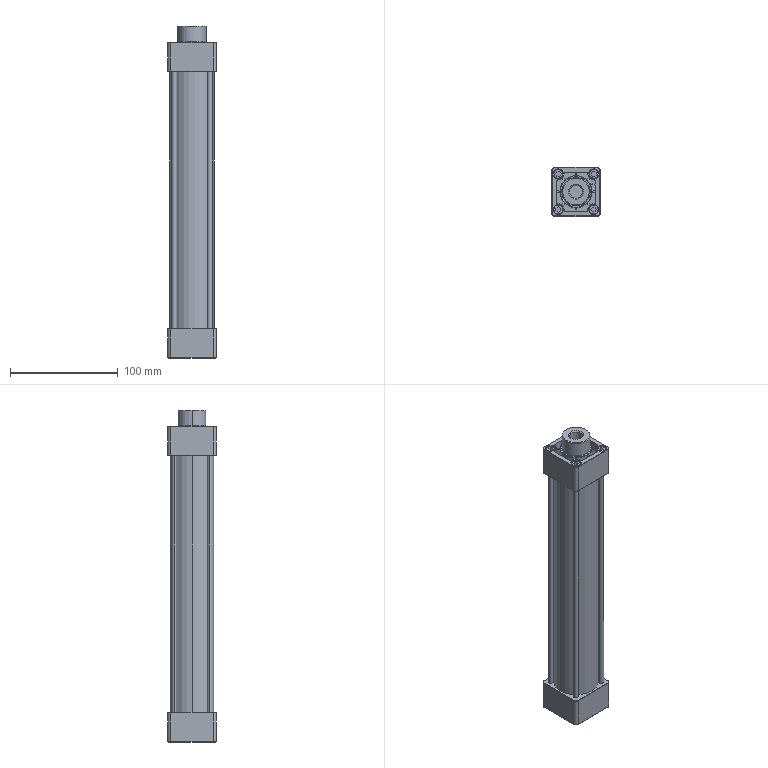Part | SolidWorks | features ICE 10, Fillet 4, Revolution 4, MirrorPattern 3, Chamfer 2, CirPattern 2, Helix 1, RevCut 1, SweepCut 1 | 2 solids | 346 faces | box 45 x 45 x 308 mm | volume 246238 mm3 | plane 162 | cylinder 112 | cone 42 | torus 26 | spline 4 | commonest cylinder face diameters 9.147 x30 8.6 x16 9 x16 2 x10 4.5 x8 6 x8